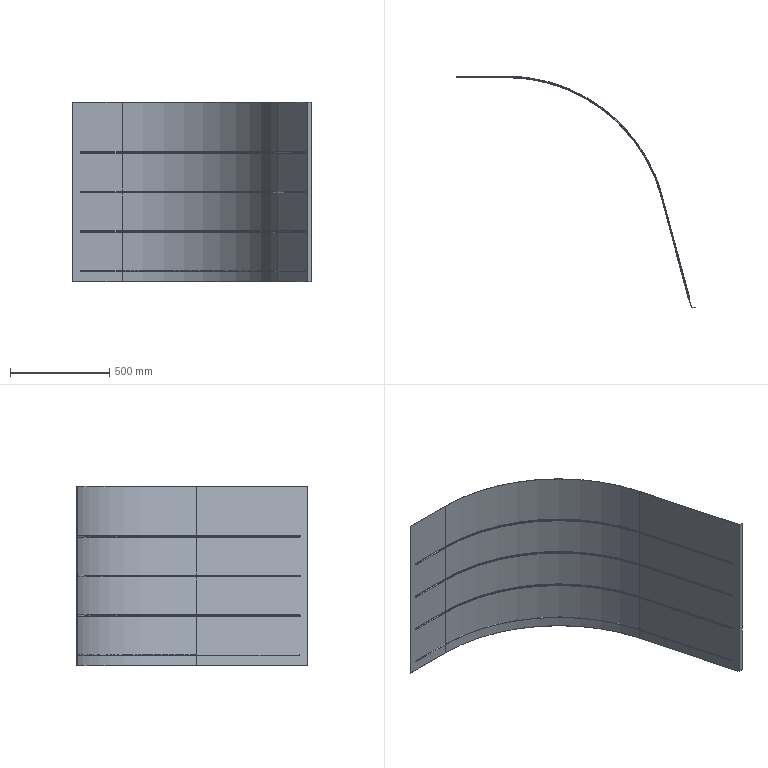Part | STEP file | 750078464 | 5 solids | 132 faces | box 1203 x 1166 x 906 mm | volume 2297945 mm3 | cylinder 64 | spline 58 | plane 10 | commonest cylinder face diameters 6 x22 2 x12 4.4 x12 8.4 x6 1622 x4 1624 x4